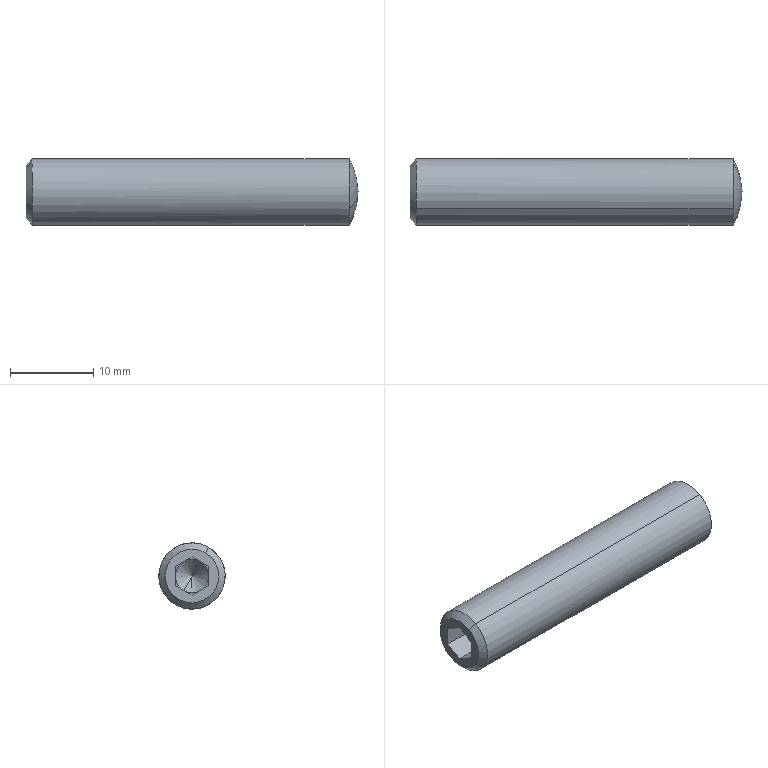Part | STEP file | SANBN8-40-Part-1-4 | 1 solid | 21 faces | box 40 x 8 x 8 mm | volume 1914 mm3 | plane 13 | cone 4 | sphere 2 | cylinder 2 | commonest cylinder face diameters 8 x2
STEP:
#1=CARTESIAN_POINT('',(8.5,0.,0.));
#2=VERTEX_POINT('',#1);
#3=CARTESIAN_POINT('',(6.5,-1.,1.732));
#4=VERTEX_POINT('',#3);
#5=CARTESIAN_POINT('',(6.5,-1.,1.732));
#6=DIRECTION('',(-0.7071,-0.3536,0.6124));
#7=VECTOR('',#6,1000.);
#8=LINE('',#5,#7);
#9=EDGE_CURVE('',#2,#4,#8,.T.);
#10=ORIENTED_EDGE('',*,*,#9,.F.);
#11=CARTESIAN_POINT('',(6.5,1.,-1.732));
#12=VERTEX_POINT('',#11);
#13=CARTESIAN_POINT('',(6.5,1.,-1.732));
#14=DIRECTION('',(-0.7071,0.3536,-0.6124));
#15=VECTOR('',#14,1000.);
#16=LINE('',#13,#15);
#17=EDGE_CURVE('',#2,#12,#16,.T.);
#18=ORIENTED_EDGE('',*,*,#17,.T.);
#19=CARTESIAN_POINT('',(6.5,-1.,-1.732));
#20=VERTEX_POINT('',#19);
#21=CARTESIAN_POINT('',(6.5,0.,0.));
#22=DIRECTION('',(-1.,0.,0.));
#23=DIRECTION('',(0.,0.5,-0.866));
#24=AXIS2_PLACEMENT_3D('',#21,#22,#23);
#25=CIRCLE('',#24,2.);
#26=EDGE_CURVE('',#12,#20,#25,.T.);
#27=ORIENTED_EDGE('',*,*,#26,.T.);
#28=CARTESIAN_POINT('',(6.5,-2.,0.));
#29=VERTEX_POINT('',#28);
#30=CARTESIAN_POINT('',(6.5,0.,0.));
#31=DIRECTION('',(-1.,0.,0.));
#32=DIRECTION('',(0.,0.5,-0.866));
#33=AXIS2_PLACEMENT_3D('',#30,#31,#32);
#34=CIRCLE('',#33,2.);
#35=EDGE_CURVE('',#20,#29,#34,.T.);
#36=ORIENTED_EDGE('',*,*,#35,.T.);
#37=CARTESIAN_POINT('',(6.5,0.,0.));
#38=DIRECTION('',(-1.,0.,0.));
#39=DIRECTION('',(0.,0.5,-0.866));
#40=AXIS2_PLACEMENT_3D('',#37,#38,#39);
#41=CIRCLE('',#40,2.);
#42=EDGE_CURVE('',#29,#4,#41,.T.);
#43=ORIENTED_EDGE('',*,*,#42,.T.);
#44=EDGE_LOOP('',(#10,#18,#27,#36,#43));
#45=FACE_OUTER_BOUND('',#44,.T.);
#46=CARTESIAN_POINT('',(6.5,0.,0.));
#47=DIRECTION('',(-1.,0.,0.));
#48=DIRECTION('',(0.,-0.5,0.866));
#49=AXIS2_PLACEMENT_3D('',#46,#47,#48);
#50=CONICAL_SURFACE('',#49,2.,0.7854);
#51=ADVANCED_FACE('',(#45),#50,.F.);
#52=CARTESIAN_POINT('',(41.428,2.,-3.464));
#53=VERTEX_POINT('',#52);
#54=CARTESIAN_POINT('',(41.428,3.464,2.));
#55=VERTEX_POINT('',#54);
#56=CARTESIAN_POINT('',(41.428,0.,0.));
#57=DIRECTION('',(1.,0.,0.));
#58=DIRECTION('',(0.,0.5,-0.866));
#59=AXIS2_PLACEMENT_3D('',#56,#57,#58);
#60=CIRCLE('',#59,4.);
#61=EDGE_CURVE('',#53,#55,#60,.T.);
#62=ORIENTED_EDGE('',*,*,#61,.T.);
#63=CARTESIAN_POINT('',(42.5,0.,0.));
#64=VERTEX_POINT('',#63);
#65=CARTESIAN_POINT('',(34.5,0.,0.));
#66=DIRECTION('',(0.,0.5,-0.866));
#67=DIRECTION('',(0.,0.866,0.5));
#68=AXIS2_PLACEMENT_3D('',#65,#66,#67);
#69=CIRCLE('',#68,8.);
#70=EDGE_CURVE('',#55,#64,#69,.T.);
#71=ORIENTED_EDGE('',*,*,#70,.T.);
#72=CARTESIAN_POINT('',(41.428,-3.464,-2.));
#73=VERTEX_POINT('',#72);
#74=CARTESIAN_POINT('',(34.5,0.,0.));
#75=DIRECTION('',(0.,-0.5,0.866));
#76=DIRECTION('',(0.,-0.866,-0.5));
#77=AXIS2_PLACEMENT_3D('',#74,#75,#76);
#78=CIRCLE('',#77,8.);
#79=EDGE_CURVE('',#73,#64,#78,.T.);
#80=ORIENTED_EDGE('',*,*,#79,.F.);
#81=CARTESIAN_POINT('',(41.428,0.,0.));
#82=DIRECTION('',(1.,0.,0.));
#83=DIRECTION('',(0.,0.5,-0.866));
#84=AXIS2_PLACEMENT_3D('',#81,#82,#83);
#85=CIRCLE('',#84,4.);
#86=EDGE_CURVE('',#73,#53,#85,.T.);
#87=ORIENTED_EDGE('',*,*,#86,.T.);
#88=EDGE_LOOP('',(#62,#71,#80,#87));
#89=FACE_OUTER_BOUND('',#88,.T.);
#90=CARTESIAN_POINT('',(34.5,0.,0.));
#91=DIRECTION('',(0.,0.5,-0.866));
#92=DIRECTION('',(0.,-0.866,-0.5));
#93=AXIS2_PLACEMENT_3D('',#90,#91,#92);
#94=SPHERICAL_SURFACE('',#93,8.);
#95=ADVANCED_FACE('',(#89),#94,.T.);
#96=CARTESIAN_POINT('',(3.267,2.,-3.464));
#97=VERTEX_POINT('',#96);
#98=CARTESIAN_POINT('',(3.267,-2.,3.464));
#99=VERTEX_POINT('',#98);
#100=CARTESIAN_POINT('',(3.267,0.,0.));
#101=DIRECTION('',(1.,0.,0.));
#102=DIRECTION('',(0.,0.5,-0.866));
#103=AXIS2_PLACEMENT_3D('',#100,#101,#102);
#104=CIRCLE('',#103,4.);
#105=EDGE_CURVE('',#97,#99,#104,.T.);
#106=ORIENTED_EDGE('',*,*,#105,.T.);
#107=CARTESIAN_POINT('',(41.428,-2.,3.464));
#108=VERTEX_POINT('',#107);
#109=CARTESIAN_POINT('',(42.5,-2.,3.464));
#110=DIRECTION('',(1.,0.,0.));
#111=VECTOR('',#110,1000.);
#112=LINE('',#109,#111);
#113=EDGE_CURVE('',#99,#108,#112,.T.);
#114=ORIENTED_EDGE('',*,*,#113,.T.);
#115=CARTESIAN_POINT('',(41.428,0.,0.));
#116=DIRECTION('',(1.,0.,0.));
#117=DIRECTION('',(0.,0.5,-0.866));
#118=AXIS2_PLACEMENT_3D('',#115,#116,#117);
#119=CIRCLE('',#118,4.);
#120=EDGE_CURVE('',#55,#108,#119,.T.);
#121=ORIENTED_EDGE('',*,*,#120,.F.);
#122=ORIENTED_EDGE('',*,*,#61,.F.);
#123=CARTESIAN_POINT('',(42.5,2.,-3.464));
#124=DIRECTION('',(1.,0.,0.));
#125=VECTOR('',#124,1000.);
#126=LINE('',#123,#125);
#127=EDGE_CURVE('',#97,#53,#126,.T.);
#128=ORIENTED_EDGE('',*,*,#127,.F.);
#129=EDGE_LOOP('',(#106,#114,#121,#122,#128));
#130=FACE_OUTER_BOUND('',#129,.T.);
#131=CARTESIAN_POINT('',(42.5,0.,0.));
#132=DIRECTION('',(1.,0.,0.));
#133=DIRECTION('',(0.,0.5,-0.866));
#134=AXIS2_PLACEMENT_3D('',#131,#132,#133);
#135=CYLINDRICAL_SURFACE('',#134,4.);
#136=ADVANCED_FACE('',(#130),#135,.T.);
#137=CARTESIAN_POINT('',(2.5,1.617,-2.8));
#138=VERTEX_POINT('',#137);
#139=CARTESIAN_POINT('',(2.5,-1.616,2.8));
#140=VERTEX_POINT('',#139);
#141=CARTESIAN_POINT('',(2.5,0.,0.));
#142=DIRECTION('',(1.,0.,0.));
#143=DIRECTION('',(0.,0.5,-0.866));
#144=AXIS2_PLACEMENT_3D('',#141,#142,#143);
#145=CIRCLE('',#144,3.233);
#146=EDGE_CURVE('',#138,#140,#145,.T.);
#147=ORIENTED_EDGE('',*,*,#146,.T.);
#148=CARTESIAN_POINT('',(2.5,-1.616,2.8));
#149=DIRECTION('',(0.7071,-0.3536,0.6124));
#150=VECTOR('',#149,1000.);
#151=LINE('',#148,#150);
#152=EDGE_CURVE('',#140,#99,#151,.T.);
#153=ORIENTED_EDGE('',*,*,#152,.T.);
#154=ORIENTED_EDGE('',*,*,#105,.F.);
#155=CARTESIAN_POINT('',(2.5,1.617,-2.8));
#156=DIRECTION('',(0.7071,0.3536,-0.6124));
#157=VECTOR('',#156,1000.);
#158=LINE('',#155,#157);
#159=EDGE_CURVE('',#138,#97,#158,.T.);
#160=ORIENTED_EDGE('',*,*,#159,.F.);
#161=EDGE_LOOP('',(#147,#153,#154,#160));
#162=FACE_OUTER_BOUND('',#161,.T.);
#163=CARTESIAN_POINT('',(2.5,0.,0.));
#164=DIRECTION('',(1.,0.,0.));
#165=DIRECTION('',(0.,0.5,-0.866));
#166=AXIS2_PLACEMENT_3D('',#163,#164,#165);
#167=CONICAL_SURFACE('',#166,3.233,0.7854);
#168=ADVANCED_FACE('',(#162),#167,.T.);
#169=ORIENTED_EDGE('',*,*,#35,.F.);
#170=CARTESIAN_POINT('',(6.5,-2.,-1.155));
#171=VERTEX_POINT('',#170);
#172=CARTESIAN_POINT('',(6.5,-2.,-1.155));
#173=DIRECTION('',(0.,0.866,-0.5));
#174=VECTOR('',#173,1000.);
#175=LINE('',#172,#174);
#176=EDGE_CURVE('',#171,#20,#175,.T.);
#177=ORIENTED_EDGE('',*,*,#176,.F.);
#178=CARTESIAN_POINT('',(6.5,-2.,1.155));
#179=DIRECTION('',(0.,0.,-1.));
#180=VECTOR('',#179,1000.);
#181=LINE('',#178,#180);
#182=EDGE_CURVE('',#29,#171,#181,.T.);
#183=ORIENTED_EDGE('',*,*,#182,.F.);
#184=EDGE_LOOP('',(#169,#177,#183));
#185=FACE_OUTER_BOUND('',#184,.T.);
#186=CARTESIAN_POINT('',(6.5,0.,0.));
#187=DIRECTION('',(1.,0.,0.));
#188=DIRECTION('',(0.,0.5,-0.866));
#189=AXIS2_PLACEMENT_3D('',#186,#187,#188);
#190=PLANE('',#189);
#191=ADVANCED_FACE('',(#185),#190,.F.);
#192=ORIENTED_EDGE('',*,*,#42,.F.);
#193=CARTESIAN_POINT('',(6.5,-2.,1.155));
#194=VERTEX_POINT('',#193);
#195=CARTESIAN_POINT('',(6.5,-2.,1.155));
#196=DIRECTION('',(0.,0.,-1.));
#197=VECTOR('',#196,1000.);
#198=LINE('',#195,#197);
#199=EDGE_CURVE('',#194,#29,#198,.T.);
#200=ORIENTED_EDGE('',*,*,#199,.F.);
#201=CARTESIAN_POINT('',(6.5,0.,2.309));
#202=DIRECTION('',(0.,-0.866,-0.5));
#203=VECTOR('',#202,1000.);
#204=LINE('',#201,#203);
#205=EDGE_CURVE('',#4,#194,#204,.T.);
#206=ORIENTED_EDGE('',*,*,#205,.F.);
#207=EDGE_LOOP('',(#192,#200,#206));
#208=FACE_OUTER_BOUND('',#207,.T.);
#209=CARTESIAN_POINT('',(6.5,0.,0.));
#210=DIRECTION('',(1.,0.,0.));
#211=DIRECTION('',(0.,0.5,-0.866));
#212=AXIS2_PLACEMENT_3D('',#209,#210,#211);
#213=PLANE('',#212);
#214=ADVANCED_FACE('',(#208),#213,.F.);
#215=CARTESIAN_POINT('',(6.5,1.,1.732));
#216=VERTEX_POINT('',#215);
#217=CARTESIAN_POINT('',(6.5,0.,0.));
#218=DIRECTION('',(-1.,0.,0.));
#219=DIRECTION('',(0.,0.5,-0.866));
#220=AXIS2_PLACEMENT_3D('',#217,#218,#219);
#221=CIRCLE('',#220,2.);
#222=EDGE_CURVE('',#4,#216,#221,.T.);
#223=ORIENTED_EDGE('',*,*,#222,.F.);
#224=CARTESIAN_POINT('',(6.5,0.,2.309));
#225=VERTEX_POINT('',#224);
#226=CARTESIAN_POINT('',(6.5,0.,2.309));
#227=DIRECTION('',(0.,-0.866,-0.5));
#228=VECTOR('',#227,1000.);
#229=LINE('',#226,#228);
#230=EDGE_CURVE('',#225,#4,#229,.T.);
#231=ORIENTED_EDGE('',*,*,#230,.F.);
#232=CARTESIAN_POINT('',(6.5,2.,1.155));
#233=DIRECTION('',(0.,-0.866,0.5));
#234=VECTOR('',#233,1000.);
#235=LINE('',#232,#234);
#236=EDGE_CURVE('',#216,#225,#235,.T.);
#237=ORIENTED_EDGE('',*,*,#236,.F.);
#238=EDGE_LOOP('',(#223,#231,#237));
#239=FACE_OUTER_BOUND('',#238,.T.);
#240=CARTESIAN_POINT('',(6.5,0.,0.));
#241=DIRECTION('',(1.,0.,0.));
#242=DIRECTION('',(0.,0.5,-0.866));
#243=AXIS2_PLACEMENT_3D('',#240,#241,#242);
#244=PLANE('',#243);
#245=ADVANCED_FACE('',(#239),#244,.F.);
#246=CARTESIAN_POINT('',(6.5,2.,0.));
#247=VERTEX_POINT('',#246);
#248=CARTESIAN_POINT('',(6.5,0.,0.));
#249=DIRECTION('',(-1.,0.,0.));
#250=DIRECTION('',(0.,0.5,-0.866));
#251=AXIS2_PLACEMENT_3D('',#248,#249,#250);
#252=CIRCLE('',#251,2.);
#253=EDGE_CURVE('',#216,#247,#252,.T.);
#254=ORIENTED_EDGE('',*,*,#253,.F.);
#255=CARTESIAN_POINT('',(6.5,2.,1.155));
#256=VERTEX_POINT('',#255);
#257=CARTESIAN_POINT('',(6.5,2.,1.155));
#258=DIRECTION('',(0.,-0.866,0.5));
#259=VECTOR('',#258,1000.);
#260=LINE('',#257,#259);
#261=EDGE_CURVE('',#256,#216,#260,.T.);
#262=ORIENTED_EDGE('',*,*,#261,.F.);
#263=CARTESIAN_POINT('',(6.5,2.,-1.155));
#264=DIRECTION('',(0.,0.,1.));
#265=VECTOR('',#264,1000.);
#266=LINE('',#263,#265);
#267=EDGE_CURVE('',#247,#256,#266,.T.);
#268=ORIENTED_EDGE('',*,*,#267,.F.);
#269=EDGE_LOOP('',(#254,#262,#268));
#270=FACE_OUTER_BOUND('',#269,.T.);
#271=CARTESIAN_POINT('',(6.5,0.,0.));
#272=DIRECTION('',(1.,0.,0.));
#273=DIRECTION('',(0.,0.5,-0.866));
#274=AXIS2_PLACEMENT_3D('',#271,#272,#273);
#275=PLANE('',#274);
#276=ADVANCED_FACE('',(#270),#275,.F.);
#277=ORIENTED_EDGE('',*,*,#26,.F.);
#278=CARTESIAN_POINT('',(6.5,0.,-2.309));
#279=VERTEX_POINT('',#278);
#280=CARTESIAN_POINT('',(6.5,0.,-2.309));
#281=DIRECTION('',(0.,0.866,0.5));
#282=VECTOR('',#281,1000.);
#283=LINE('',#280,#282);
#284=EDGE_CURVE('',#279,#12,#283,.T.);
#285=ORIENTED_EDGE('',*,*,#284,.F.);
#286=CARTESIAN_POINT('',(6.5,-2.,-1.155));
#287=DIRECTION('',(0.,0.866,-0.5));
#288=VECTOR('',#287,1000.);
#289=LINE('',#286,#288);
#290=EDGE_CURVE('',#20,#279,#289,.T.);
#291=ORIENTED_EDGE('',*,*,#290,.F.);
#292=EDGE_LOOP('',(#277,#285,#291));
#293=FACE_OUTER_BOUND('',#292,.T.);
#294=CARTESIAN_POINT('',(6.5,0.,0.));
#295=DIRECTION('',(1.,0.,0.));
#296=DIRECTION('',(0.,0.5,-0.866));
#297=AXIS2_PLACEMENT_3D('',#294,#295,#296);
#298=PLANE('',#297);
#299=ADVANCED_FACE('',(#293),#298,.F.);
#300=ORIENTED_EDGE('',*,*,#146,.F.);
#301=CARTESIAN_POINT('',(2.5,0.,0.));
#302=DIRECTION('',(1.,0.,0.));
#303=DIRECTION('',(0.,0.5,-0.866));
#304=AXIS2_PLACEMENT_3D('',#301,#302,#303);
#305=CIRCLE('',#304,3.233);
#306=EDGE_CURVE('',#140,#138,#305,.T.);
#307=ORIENTED_EDGE('',*,*,#306,.F.);
#308=EDGE_LOOP('',(#300,#307));
#309=FACE_OUTER_BOUND('',#308,.T.);
#310=CARTESIAN_POINT('',(2.5,0.,2.309));
#311=VERTEX_POINT('',#310);
#312=CARTESIAN_POINT('',(2.5,-2.,1.155));
#313=VERTEX_POINT('',#312);
#314=CARTESIAN_POINT('',(2.5,0.,2.309));
#315=DIRECTION('',(0.,-0.866,-0.5));
#316=VECTOR('',#315,1000.);
#317=LINE('',#314,#316);
#318=EDGE_CURVE('',#311,#313,#317,.T.);
#319=ORIENTED_EDGE('',*,*,#318,.T.);
#320=CARTESIAN_POINT('',(2.5,-2.,-1.155));
#321=VERTEX_POINT('',#320);
#322=CARTESIAN_POINT('',(2.5,-2.,1.155));
#323=DIRECTION('',(0.,0.,-1.));
#324=VECTOR('',#323,1000.);
#325=LINE('',#322,#324);
#326=EDGE_CURVE('',#313,#321,#325,.T.);
#327=ORIENTED_EDGE('',*,*,#326,.T.);
#328=CARTESIAN_POINT('',(2.5,0.,-2.309));
#329=VERTEX_POINT('',#328);
#330=CARTESIAN_POINT('',(2.5,-2.,-1.155));
#331=DIRECTION('',(0.,0.866,-0.5));
#332=VECTOR('',#331,1000.);
#333=LINE('',#330,#332);
#334=EDGE_CURVE('',#321,#329,#333,.T.);
#335=ORIENTED_EDGE('',*,*,#334,.T.);
#336=CARTESIAN_POINT('',(2.5,2.,-1.155));
#337=VERTEX_POINT('',#336);
#338=CARTESIAN_POINT('',(2.5,0.,-2.309));
#339=DIRECTION('',(0.,0.866,0.5));
#340=VECTOR('',#339,1000.);
#341=LINE('',#338,#340);
#342=EDGE_CURVE('',#329,#337,#341,.T.);
#343=ORIENTED_EDGE('',*,*,#342,.T.);
#344=CARTESIAN_POINT('',(2.5,2.,1.155));
#345=VERTEX_POINT('',#344);
#346=CARTESIAN_POINT('',(2.5,2.,-1.155));
#347=DIRECTION('',(0.,0.,1.));
#348=VECTOR('',#347,1000.);
#349=LINE('',#346,#348);
#350=EDGE_CURVE('',#337,#345,#349,.T.);
#351=ORIENTED_EDGE('',*,*,#350,.T.);
#352=CARTESIAN_POINT('',(2.5,2.,1.155));
#353=DIRECTION('',(0.,-0.866,0.5));
#354=VECTOR('',#353,1000.);
#355=LINE('',#352,#354);
#356=EDGE_CURVE('',#345,#311,#355,.T.);
#357=ORIENTED_EDGE('',*,*,#356,.T.);
#358=EDGE_LOOP('',(#319,#327,#335,#343,#351,#357));
#359=FACE_BOUND('',#358,.T.);
#360=CARTESIAN_POINT('',(2.5,0.,0.));
#361=DIRECTION('',(1.,0.,0.));
#362=DIRECTION('',(0.,0.5,-0.866));
#363=AXIS2_PLACEMENT_3D('',#360,#361,#362);
#364=PLANE('',#363);
#365=ADVANCED_FACE('',(#309,#359),#364,.F.);
#366=ORIENTED_EDGE('',*,*,#152,.F.);
#367=ORIENTED_EDGE('',*,*,#306,.T.);
#368=ORIENTED_EDGE('',*,*,#159,.T.);
#369=CARTESIAN_POINT('',(3.267,0.,0.));
#370=DIRECTION('',(1.,0.,0.));
#371=DIRECTION('',(0.,0.5,-0.866));
#372=AXIS2_PLACEMENT_3D('',#369,#370,#371);
#373=CIRCLE('',#372,4.);
#374=EDGE_CURVE('',#99,#97,#373,.T.);
#375=ORIENTED_EDGE('',*,*,#374,.F.);
#376=EDGE_LOOP('',(#366,#367,#368,#375));
#377=FACE_OUTER_BOUND('',#376,.T.);
#378=CARTESIAN_POINT('',(2.5,0.,0.));
#379=DIRECTION('',(1.,0.,0.));
#380=DIRECTION('',(0.,0.5,-0.866));
#381=AXIS2_PLACEMENT_3D('',#378,#379,#380);
#382=CONICAL_SURFACE('',#381,3.233,0.7854);
#383=ADVANCED_FACE('',(#377),#382,.T.);
#384=ORIENTED_EDGE('',*,*,#113,.F.);
#385=ORIENTED_EDGE('',*,*,#374,.T.);
#386=ORIENTED_EDGE('',*,*,#127,.T.);
#387=ORIENTED_EDGE('',*,*,#86,.F.);
#388=CARTESIAN_POINT('',(41.428,0.,0.));
#389=DIRECTION('',(1.,0.,0.));
#390=DIRECTION('',(0.,0.5,-0.866));
#391=AXIS2_PLACEMENT_3D('',#388,#389,#390);
#392=CIRCLE('',#391,4.);
#393=EDGE_CURVE('',#108,#73,#392,.T.);
#394=ORIENTED_EDGE('',*,*,#393,.F.);
#395=EDGE_LOOP('',(#384,#385,#386,#387,#394));
#396=FACE_OUTER_BOUND('',#395,.T.);
#397=CARTESIAN_POINT('',(42.5,0.,0.));
#398=DIRECTION('',(1.,0.,0.));
#399=DIRECTION('',(0.,0.5,-0.866));
#400=AXIS2_PLACEMENT_3D('',#397,#398,#399);
#401=CYLINDRICAL_SURFACE('',#400,4.);
#402=ADVANCED_FACE('',(#396),#401,.T.);
#403=ORIENTED_EDGE('',*,*,#70,.F.);
#404=ORIENTED_EDGE('',*,*,#120,.T.);
#405=ORIENTED_EDGE('',*,*,#393,.T.);
#406=ORIENTED_EDGE('',*,*,#79,.T.);
#407=EDGE_LOOP('',(#403,#404,#405,#406));
#408=FACE_OUTER_BOUND('',#407,.T.);
#409=CARTESIAN_POINT('',(34.5,0.,0.));
#410=DIRECTION('',(0.,0.5,-0.866));
#411=DIRECTION('',(0.,-0.866,-0.5));
#412=AXIS2_PLACEMENT_3D('',#409,#410,#411);
#413=SPHERICAL_SURFACE('',#412,8.);
#414=ADVANCED_FACE('',(#408),#413,.T.);
#415=ORIENTED_EDGE('',*,*,#318,.F.);
#416=CARTESIAN_POINT('',(6.5,0.,2.309));
#417=DIRECTION('',(-1.,0.,0.));
#418=VECTOR('',#417,1000.);
#419=LINE('',#416,#418);
#420=EDGE_CURVE('',#225,#311,#419,.T.);
#421=ORIENTED_EDGE('',*,*,#420,.F.);
#422=ORIENTED_EDGE('',*,*,#230,.T.);
#423=ORIENTED_EDGE('',*,*,#205,.T.);
#424=CARTESIAN_POINT('',(6.5,-2.,1.155));
#425=DIRECTION('',(-1.,0.,0.));
#426=VECTOR('',#425,1000.);
#427=LINE('',#424,#426);
#428=EDGE_CURVE('',#194,#313,#427,.T.);
#429=ORIENTED_EDGE('',*,*,#428,.T.);
#430=EDGE_LOOP('',(#415,#421,#422,#423,#429));
#431=FACE_OUTER_BOUND('',#430,.T.);
#432=CARTESIAN_POINT('',(6.5,0.,2.309));
#433=DIRECTION('',(0.,0.5,-0.866));
#434=DIRECTION('',(-1.,0.,0.));
#435=AXIS2_PLACEMENT_3D('',#432,#433,#434);
#436=PLANE('',#435);
#437=ADVANCED_FACE('',(#431),#436,.T.);
#438=ORIENTED_EDGE('',*,*,#326,.F.);
#439=ORIENTED_EDGE('',*,*,#428,.F.);
#440=ORIENTED_EDGE('',*,*,#199,.T.);
#441=ORIENTED_EDGE('',*,*,#182,.T.);
#442=CARTESIAN_POINT('',(6.5,-2.,-1.155));
#443=DIRECTION('',(-1.,0.,0.));
#444=VECTOR('',#443,1000.);
#445=LINE('',#442,#444);
#446=EDGE_CURVE('',#171,#321,#445,.T.);
#447=ORIENTED_EDGE('',*,*,#446,.T.);
#448=EDGE_LOOP('',(#438,#439,#440,#441,#447));
#449=FACE_OUTER_BOUND('',#448,.T.);
#450=CARTESIAN_POINT('',(6.5,-2.,1.155));
#451=DIRECTION('',(0.,1.,0.));
#452=DIRECTION('',(0.,0.,1.));
#453=AXIS2_PLACEMENT_3D('',#450,#451,#452);
#454=PLANE('',#453);
#455=ADVANCED_FACE('',(#449),#454,.T.);
#456=ORIENTED_EDGE('',*,*,#334,.F.);
#457=ORIENTED_EDGE('',*,*,#446,.F.);
#458=ORIENTED_EDGE('',*,*,#176,.T.);
#459=ORIENTED_EDGE('',*,*,#290,.T.);
#460=CARTESIAN_POINT('',(6.5,0.,-2.309));
#461=DIRECTION('',(-1.,0.,0.));
#462=VECTOR('',#461,1000.);
#463=LINE('',#460,#462);
#464=EDGE_CURVE('',#279,#329,#463,.T.);
#465=ORIENTED_EDGE('',*,*,#464,.T.);
#466=EDGE_LOOP('',(#456,#457,#458,#459,#465));
#467=FACE_OUTER_BOUND('',#466,.T.);
#468=CARTESIAN_POINT('',(6.5,-2.,-1.155));
#469=DIRECTION('',(0.,0.5,0.866));
#470=DIRECTION('',(0.,-0.866,0.5));
#471=AXIS2_PLACEMENT_3D('',#468,#469,#470);
#472=PLANE('',#471);
#473=ADVANCED_FACE('',(#467),#472,.T.);
#474=ORIENTED_EDGE('',*,*,#342,.F.);
#475=ORIENTED_EDGE('',*,*,#464,.F.);
#476=ORIENTED_EDGE('',*,*,#284,.T.);
#477=CARTESIAN_POINT('',(6.5,2.,-1.155));
#478=VERTEX_POINT('',#477);
#479=CARTESIAN_POINT('',(6.5,0.,-2.309));
#480=DIRECTION('',(0.,0.866,0.5));
#481=VECTOR('',#480,1000.);
#482=LINE('',#479,#481);
#483=EDGE_CURVE('',#12,#478,#482,.T.);
#484=ORIENTED_EDGE('',*,*,#483,.T.);
#485=CARTESIAN_POINT('',(6.5,2.,-1.155));
#486=DIRECTION('',(-1.,0.,0.));
#487=VECTOR('',#486,1000.);
#488=LINE('',#485,#487);
#489=EDGE_CURVE('',#478,#337,#488,.T.);
#490=ORIENTED_EDGE('',*,*,#489,.T.);
#491=EDGE_LOOP('',(#474,#475,#476,#484,#490));
#492=FACE_OUTER_BOUND('',#491,.T.);
#493=CARTESIAN_POINT('',(6.5,0.,-2.309));
#494=DIRECTION('',(0.,-0.5,0.866));
#495=DIRECTION('',(1.,0.,0.));
#496=AXIS2_PLACEMENT_3D('',#493,#494,#495);
#497=PLANE('',#496);
#498=ADVANCED_FACE('',(#492),#497,.T.);
#499=ORIENTED_EDGE('',*,*,#350,.F.);
#500=ORIENTED_EDGE('',*,*,#489,.F.);
#501=CARTESIAN_POINT('',(6.5,2.,-1.155));
#502=DIRECTION('',(0.,0.,1.));
#503=VECTOR('',#502,1000.);
#504=LINE('',#501,#503);
#505=EDGE_CURVE('',#478,#247,#504,.T.);
#506=ORIENTED_EDGE('',*,*,#505,.T.);
#507=ORIENTED_EDGE('',*,*,#267,.T.);
#508=CARTESIAN_POINT('',(6.5,2.,1.155));
#509=DIRECTION('',(-1.,0.,0.));
#510=VECTOR('',#509,1000.);
#511=LINE('',#508,#510);
#512=EDGE_CURVE('',#256,#345,#511,.T.);
#513=ORIENTED_EDGE('',*,*,#512,.T.);
#514=EDGE_LOOP('',(#499,#500,#506,#507,#513));
#515=FACE_OUTER_BOUND('',#514,.T.);
#516=CARTESIAN_POINT('',(6.5,2.,-1.155));
#517=DIRECTION('',(0.,-1.,0.));
#518=DIRECTION('',(0.,0.,-1.));
#519=AXIS2_PLACEMENT_3D('',#516,#517,#518);
#520=PLANE('',#519);
#521=ADVANCED_FACE('',(#515),#520,.T.);
#522=ORIENTED_EDGE('',*,*,#356,.F.);
#523=ORIENTED_EDGE('',*,*,#512,.F.);
#524=ORIENTED_EDGE('',*,*,#261,.T.);
#525=ORIENTED_EDGE('',*,*,#236,.T.);
#526=ORIENTED_EDGE('',*,*,#420,.T.);
#527=EDGE_LOOP('',(#522,#523,#524,#525,#526));
#528=FACE_OUTER_BOUND('',#527,.T.);
#529=CARTESIAN_POINT('',(6.5,2.,1.155));
#530=DIRECTION('',(0.,-0.5,-0.866));
#531=DIRECTION('',(0.,0.866,-0.5));
#532=AXIS2_PLACEMENT_3D('',#529,#530,#531);
#533=PLANE('',#532);
#534=ADVANCED_FACE('',(#528),#533,.T.);
#535=CARTESIAN_POINT('',(6.5,0.,0.));
#536=DIRECTION('',(-1.,0.,0.));
#537=DIRECTION('',(0.,0.5,-0.866));
#538=AXIS2_PLACEMENT_3D('',#535,#536,#537);
#539=CIRCLE('',#538,2.);
#540=EDGE_CURVE('',#247,#12,#539,.T.);
#541=ORIENTED_EDGE('',*,*,#540,.F.);
#542=ORIENTED_EDGE('',*,*,#505,.F.);
#543=ORIENTED_EDGE('',*,*,#483,.F.);
#544=EDGE_LOOP('',(#541,#542,#543));
#545=FACE_OUTER_BOUND('',#544,.T.);
#546=CARTESIAN_POINT('',(6.5,0.,0.));
#547=DIRECTION('',(1.,0.,0.));
#548=DIRECTION('',(0.,0.5,-0.866));
#549=AXIS2_PLACEMENT_3D('',#546,#547,#548);
#550=PLANE('',#549);
#551=ADVANCED_FACE('',(#545),#550,.F.);
#552=ORIENTED_EDGE('',*,*,#17,.F.);
#553=ORIENTED_EDGE('',*,*,#9,.T.);
#554=ORIENTED_EDGE('',*,*,#222,.T.);
#555=ORIENTED_EDGE('',*,*,#253,.T.);
#556=ORIENTED_EDGE('',*,*,#540,.T.);
#557=EDGE_LOOP('',(#552,#553,#554,#555,#556));
#558=FACE_OUTER_BOUND('',#557,.T.);
#559=CARTESIAN_POINT('',(6.5,0.,0.));
#560=DIRECTION('',(-1.,0.,0.));
#561=DIRECTION('',(0.,-0.5,0.866));
#562=AXIS2_PLACEMENT_3D('',#559,#560,#561);
#563=CONICAL_SURFACE('',#562,2.,0.7854);
#564=ADVANCED_FACE('',(#558),#563,.F.);
#565=CLOSED_SHELL('',(#51,#95,#136,#168,#191,#214,#245,#276,#299,#365,#383,#402,#414,#437,#455,#473,#498,#521,#534,#551,#564));
#566=MANIFOLD_SOLID_BREP('',#565);
#567=CARTESIAN_POINT('',(0.,0.,0.));
#568=DIRECTION('',(0.,0.,1.));
#569=DIRECTION('',(1.,0.,0.));
#570=AXIS2_PLACEMENT_3D('',#567,#568,#569);
#571=(LENGTH_UNIT()NAMED_UNIT(*)SI_UNIT(.MILLI.,.METRE.));
#572=UNCERTAINTY_MEASURE_WITH_UNIT(LENGTH_MEASURE(0.00001),#571,'','');
#573=(NAMED_UNIT(*)PLANE_ANGLE_UNIT()SI_UNIT($,.RADIAN.));
#574=(NAMED_UNIT(*)SI_UNIT($,.STERADIAN.)SOLID_ANGLE_UNIT());
#575=(GEOMETRIC_REPRESENTATION_CONTEXT(3)GLOBAL_UNCERTAINTY_ASSIGNED_CONTEXT((#572))GLOBAL_UNIT_ASSIGNED_CONTEXT((#571,#573,#574))REPRESENTATION_CONTEXT('',''));
#576=ADVANCED_BREP_SHAPE_REPRESENTATION('',(#566,#570),#575);